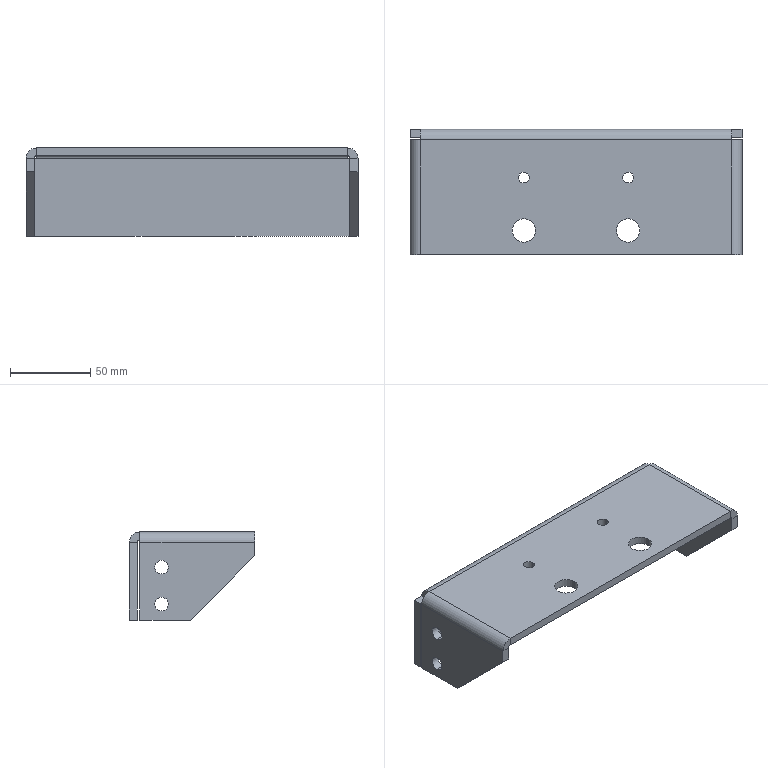Part | STEP file | Limit fixing plate 2 | 1 solid | 50 faces | box 207 x 78 x 55 mm | volume 153668 mm3 | plane 28 | cylinder 22 | commonest cylinder face diameters 8.5 x8 6.8 x4 14.5 x4 3 x3 13 x3